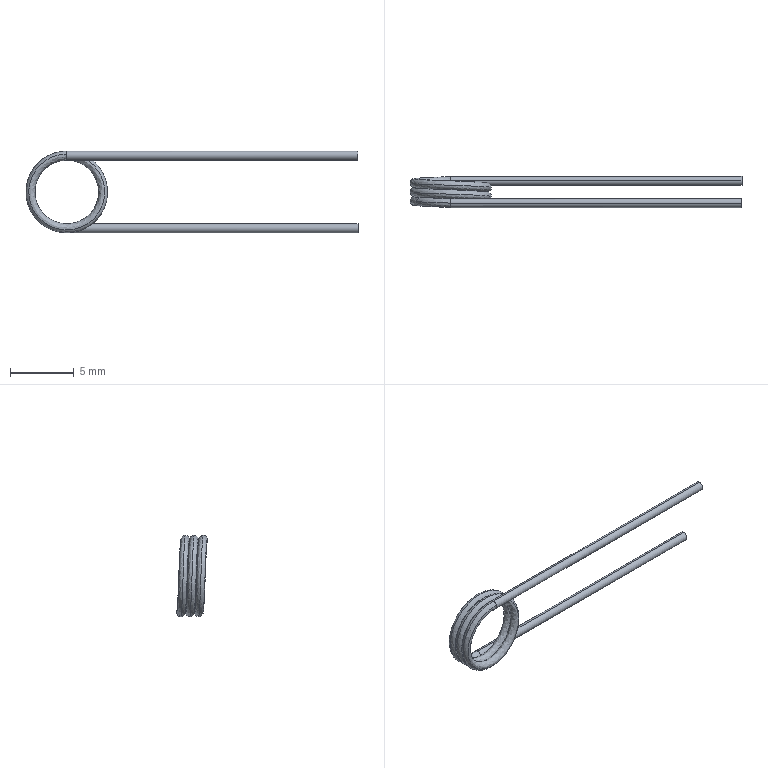Part | SolidWorks | features CompositeCurve 1, Helix 1, MoveFace 1, Sweep 1 | 1 solid | 9 faces | box 26.05 x 2.45 x 6.4 mm | volume 34.304 mm3 | cylinder 4 | spline 3 | plane 2 | commonest cylinder face diameters 0.7 x4
STEP:
#1=CARTESIAN_POINT('',(22.85,1.75,-3.2));
#2=VERTEX_POINT('',#1);
#3=CARTESIAN_POINT('',(22.85,1.75,-2.5));
#4=VERTEX_POINT('',#3);
#5=CARTESIAN_POINT('',(22.85,1.75,-2.85));
#6=DIRECTION('',(1.,0.,0.));
#7=DIRECTION('',(0.,0.00009155,-1.));
#8=AXIS2_PLACEMENT_3D('',#5,#6,#7);
#9=CIRCLE('',#8,0.35);
#10=EDGE_CURVE('',#2,#4,#9,.T.);
#11=ORIENTED_EDGE('',*,*,#10,.F.);
#12=CARTESIAN_POINT('',(-0.000000536,1.75,-3.2));
#13=VERTEX_POINT('',#12);
#14=CARTESIAN_POINT('',(12.85,1.75,-3.2));
#15=DIRECTION('',(-1.,0.,0.));
#16=VECTOR('',#15,1000.);
#17=LINE('',#14,#16);
#18=EDGE_CURVE('',#2,#13,#17,.T.);
#19=ORIENTED_EDGE('',*,*,#18,.T.);
#20=CARTESIAN_POINT('',(-0.006305,2.074,-2.979));
#21=VERTEX_POINT('',#20);
#22=CARTESIAN_POINT('',(0.,1.75,-2.85));
#23=DIRECTION('',(1.,0.,0.));
#24=DIRECTION('',(0.,0.00009155,-1.));
#25=AXIS2_PLACEMENT_3D('',#22,#23,#24);
#26=CIRCLE('',#25,0.35);
#27=EDGE_CURVE('',#13,#21,#26,.T.);
#28=ORIENTED_EDGE('',*,*,#27,.T.);
#29=CARTESIAN_POINT('',(0.,1.75,-2.5));
#30=VERTEX_POINT('',#29);
#31=CARTESIAN_POINT('',(0.,1.75,-2.85));
#32=DIRECTION('',(1.,0.,0.));
#33=DIRECTION('',(0.,0.00009155,-1.));
#34=AXIS2_PLACEMENT_3D('',#31,#32,#33);
#35=CIRCLE('',#34,0.35);
#36=EDGE_CURVE('',#21,#30,#35,.T.);
#37=ORIENTED_EDGE('',*,*,#36,.T.);
#38=CARTESIAN_POINT('',(12.85,1.75,-2.5));
#39=DIRECTION('',(-1.,0.,0.));
#40=VECTOR('',#39,1000.);
#41=LINE('',#38,#40);
#42=EDGE_CURVE('',#4,#30,#41,.T.);
#43=ORIENTED_EDGE('',*,*,#42,.F.);
#44=EDGE_LOOP('',(#11,#19,#28,#37,#43));
#45=FACE_OUTER_BOUND('',#44,.T.);
#46=CARTESIAN_POINT('',(12.85,1.75,-2.85));
#47=DIRECTION('',(-1.,0.,0.));
#48=DIRECTION('',(0.,0.,1.));
#49=AXIS2_PLACEMENT_3D('',#46,#47,#48);
#50=CYLINDRICAL_SURFACE('',#49,0.35);
#51=ADVANCED_FACE('',(#45),#50,.T.);
#52=CARTESIAN_POINT('',(0.006305,0.3239,2.979));
#53=VERTEX_POINT('',#52);
#54=CARTESIAN_POINT('',(0.,0.,3.2));
#55=VERTEX_POINT('',#54);
#56=CARTESIAN_POINT('',(0.006305,0.3239,2.979));
#57=CARTESIAN_POINT('',(0.01048,0.2681,3.104));
#58=CARTESIAN_POINT('',(0.005425,0.1388,3.2));
#59=CARTESIAN_POINT('',(0.,0.,3.2));
#60=B_SPLINE_CURVE_WITH_KNOTS('',3,(#56,#57,#58,#59),.UNSPECIFIED.,.F.,.F.,(4,4),(0.00002721,0.1895),.UNSPECIFIED.);
#61=EDGE_CURVE('',#53,#55,#60,.T.);
#62=ORIENTED_EDGE('',*,*,#61,.T.);
#63=CARTESIAN_POINT('',(22.85,0.,3.2));
#64=VERTEX_POINT('',#63);
#65=CARTESIAN_POINT('',(0.,0.,3.2));
#66=DIRECTION('',(1.,0.,0.));
#67=VECTOR('',#66,1000.);
#68=LINE('',#65,#67);
#69=EDGE_CURVE('',#55,#64,#68,.T.);
#70=ORIENTED_EDGE('',*,*,#69,.T.);
#71=CARTESIAN_POINT('',(22.85,0.,2.5));
#72=VERTEX_POINT('',#71);
#73=CARTESIAN_POINT('',(22.85,0.,2.85));
#74=DIRECTION('',(-1.,0.,0.));
#75=DIRECTION('',(0.,0.,1.));
#76=AXIS2_PLACEMENT_3D('',#73,#74,#75);
#77=CIRCLE('',#76,0.35);
#78=EDGE_CURVE('',#64,#72,#77,.T.);
#79=ORIENTED_EDGE('',*,*,#78,.T.);
#80=CARTESIAN_POINT('',(0.,0.,2.5));
#81=VERTEX_POINT('',#80);
#82=CARTESIAN_POINT('',(0.,0.,2.5));
#83=DIRECTION('',(1.,0.,0.));
#84=VECTOR('',#83,1000.);
#85=LINE('',#82,#84);
#86=EDGE_CURVE('',#81,#72,#85,.T.);
#87=ORIENTED_EDGE('',*,*,#86,.F.);
#88=CARTESIAN_POINT('',(0.,0.,2.85));
#89=DIRECTION('',(-1.,0.,0.));
#90=DIRECTION('',(0.,0.,1.));
#91=AXIS2_PLACEMENT_3D('',#88,#89,#90);
#92=CIRCLE('',#91,0.35);
#93=EDGE_CURVE('',#53,#81,#92,.T.);
#94=ORIENTED_EDGE('',*,*,#93,.F.);
#95=EDGE_LOOP('',(#62,#70,#79,#87,#94));
#96=FACE_OUTER_BOUND('',#95,.T.);
#97=CARTESIAN_POINT('',(0.,0.,2.85));
#98=DIRECTION('',(1.,0.,0.));
#99=DIRECTION('',(0.,0.,-1.));
#100=AXIS2_PLACEMENT_3D('',#97,#98,#99);
#101=CYLINDRICAL_SURFACE('',#100,0.35);
#102=ADVANCED_FACE('',(#96),#101,.T.);
#103=ORIENTED_EDGE('',*,*,#18,.F.);
#104=CARTESIAN_POINT('',(22.85,1.75,-2.85));
#105=DIRECTION('',(1.,0.,0.));
#106=DIRECTION('',(0.,0.00009155,-1.));
#107=AXIS2_PLACEMENT_3D('',#104,#105,#106);
#108=CIRCLE('',#107,0.35);
#109=EDGE_CURVE('',#4,#2,#108,.T.);
#110=ORIENTED_EDGE('',*,*,#109,.F.);
#111=ORIENTED_EDGE('',*,*,#42,.T.);
#112=CARTESIAN_POINT('',(0.006304,1.426,-2.979));
#113=VERTEX_POINT('',#112);
#114=CARTESIAN_POINT('',(0.,1.75,-2.85));
#115=DIRECTION('',(1.,0.,0.));
#116=DIRECTION('',(0.,0.00009155,-1.));
#117=AXIS2_PLACEMENT_3D('',#114,#115,#116);
#118=CIRCLE('',#117,0.35);
#119=EDGE_CURVE('',#30,#113,#118,.T.);
#120=ORIENTED_EDGE('',*,*,#119,.T.);
#121=CARTESIAN_POINT('',(0.,1.75,-2.85));
#122=DIRECTION('',(1.,0.,0.));
#123=DIRECTION('',(0.,0.00009155,-1.));
#124=AXIS2_PLACEMENT_3D('',#121,#122,#123);
#125=CIRCLE('',#124,0.35);
#126=EDGE_CURVE('',#113,#13,#125,.T.);
#127=ORIENTED_EDGE('',*,*,#126,.T.);
#128=EDGE_LOOP('',(#103,#110,#111,#120,#127));
#129=FACE_OUTER_BOUND('',#128,.T.);
#130=CARTESIAN_POINT('',(12.85,1.75,-2.85));
#131=DIRECTION('',(-1.,0.,0.));
#132=DIRECTION('',(0.,0.,1.));
#133=AXIS2_PLACEMENT_3D('',#130,#131,#132);
#134=CYLINDRICAL_SURFACE('',#133,0.35);
#135=ADVANCED_FACE('',(#129),#134,.T.);
#136=ORIENTED_EDGE('',*,*,#36,.F.);
#137=CARTESIAN_POINT('',(0.006305,0.3239,2.979));
#138=CARTESIAN_POINT('',(-0.7712,0.3519,2.981));
#139=CARTESIAN_POINT('',(-1.545,0.381,2.663));
#140=CARTESIAN_POINT('',(-2.649,0.4392,1.566));
#141=CARTESIAN_POINT('',(-2.975,0.4683,0.7939));
#142=CARTESIAN_POINT('',(-2.98,0.5195,-0.5733));
#143=CARTESIAN_POINT('',(-2.806,0.5413,-1.156));
#144=CARTESIAN_POINT('',(-2.162,0.585,-2.13));
#145=CARTESIAN_POINT('',(-1.69,0.6069,-2.521));
#146=CARTESIAN_POINT('',(-0.4324,0.658,-3.048));
#147=CARTESIAN_POINT('',(0.405,0.6871,-3.052));
#148=CARTESIAN_POINT('',(1.67,0.7383,-2.534));
#149=CARTESIAN_POINT('',(2.142,0.7601,-2.15));
#150=CARTESIAN_POINT('',(2.795,0.8037,-1.182));
#151=CARTESIAN_POINT('',(2.976,0.8257,-0.5972));
#152=CARTESIAN_POINT('',(2.981,0.8768,0.7668));
#153=CARTESIAN_POINT('',(2.665,0.9058,1.542));
#154=CARTESIAN_POINT('',(1.702,0.957,2.513));
#155=CARTESIAN_POINT('',(1.167,0.9788,2.801));
#156=CARTESIAN_POINT('',(0.02248,1.022,3.035));
#157=CARTESIAN_POINT('',(-0.587,1.044,2.978));
#158=CARTESIAN_POINT('',(-1.849,1.096,2.461));
#159=CARTESIAN_POINT('',(-2.445,1.125,1.872));
#160=CARTESIAN_POINT('',(-2.973,1.176,0.6109));
#161=CARTESIAN_POINT('',(-3.035,1.198,0.005944));
#162=CARTESIAN_POINT('',(-2.812,1.241,-1.14));
#163=CARTESIAN_POINT('',(-2.526,1.263,-1.682));
#164=CARTESIAN_POINT('',(-1.566,1.314,-2.65));
#165=CARTESIAN_POINT('',(-0.7938,1.343,-2.975));
#166=CARTESIAN_POINT('',(0.5733,1.395,-2.98));
#167=CARTESIAN_POINT('',(1.156,1.416,-2.806));
#168=CARTESIAN_POINT('',(2.13,1.46,-2.162));
#169=CARTESIAN_POINT('',(2.521,1.482,-1.69));
#170=CARTESIAN_POINT('',(3.048,1.533,-0.4324));
#171=CARTESIAN_POINT('',(3.052,1.562,0.405));
#172=CARTESIAN_POINT('',(2.534,1.613,1.67));
#173=CARTESIAN_POINT('',(2.15,1.635,2.142));
#174=CARTESIAN_POINT('',(1.182,1.679,2.795));
#175=CARTESIAN_POINT('',(0.5972,1.701,2.976));
#176=CARTESIAN_POINT('',(-0.7668,1.752,2.981));
#177=CARTESIAN_POINT('',(-1.542,1.781,2.665));
#178=CARTESIAN_POINT('',(-2.513,1.832,1.702));
#179=CARTESIAN_POINT('',(-2.801,1.854,1.167));
#180=CARTESIAN_POINT('',(-3.034,1.897,0.0225));
#181=CARTESIAN_POINT('',(-2.978,1.919,-0.587));
#182=CARTESIAN_POINT('',(-2.46,1.971,-1.85));
#183=CARTESIAN_POINT('',(-1.872,2.,-2.445));
#184=CARTESIAN_POINT('',(-0.7917,2.043,-2.897));
#185=CARTESIAN_POINT('',(-0.4042,2.058,-2.976));
#186=CARTESIAN_POINT('',(-0.006305,2.074,-2.979));
#187=B_SPLINE_CURVE_WITH_KNOTS('',3,(#137,#138,#139,#140,#141,#142,#143,#144,#145,#146,#147,#148,#149,#150,#151,#152,#153,#154,#155,#156,#157,#158,#159,#160,#161,#162,#163,#164,#165,#166,#167,#168,#169,#170,#171,#172,#173,#174,#175,#176,#177,#178,#179,#180,#181,#182,#183,#184,#185,#186),.UNSPECIFIED.,.F.,.F.,(4,2,2,2,2,2,2,2,2,2,2,2,2,2,2,2,2,2,2,2,2,2,2,2,4),(0.,0.04998,0.09999,0.1375,0.175,0.225,0.2625,0.3,0.35,0.3875,0.425,0.475,0.5125,0.55,0.6,0.6375,0.675,0.725,0.7625,0.8,0.85,0.8875,0.925,0.975,1.),.UNSPECIFIED.);
#188=EDGE_CURVE('',#53,#21,#187,.T.);
#189=ORIENTED_EDGE('',*,*,#188,.F.);
#190=ORIENTED_EDGE('',*,*,#93,.T.);
#191=CARTESIAN_POINT('',(-0.006304,-0.3239,2.979));
#192=VERTEX_POINT('',#191);
#193=CARTESIAN_POINT('',(0.,0.,2.85));
#194=DIRECTION('',(-1.,0.,0.));
#195=DIRECTION('',(0.,0.,1.));
#196=AXIS2_PLACEMENT_3D('',#193,#194,#195);
#197=CIRCLE('',#196,0.35);
#198=EDGE_CURVE('',#81,#192,#197,.T.);
#199=ORIENTED_EDGE('',*,*,#198,.T.);
#200=CARTESIAN_POINT('',(0.006304,1.426,-2.979));
#201=CARTESIAN_POINT('',(-0.379,1.413,-2.98));
#202=CARTESIAN_POINT('',(-0.7673,1.398,-2.904));
#203=CARTESIAN_POINT('',(-1.851,1.354,-2.461));
#204=CARTESIAN_POINT('',(-2.445,1.325,-1.871));
#205=CARTESIAN_POINT('',(-2.973,1.274,-0.6122));
#206=CARTESIAN_POINT('',(-3.035,1.252,-0.003211));
#207=CARTESIAN_POINT('',(-2.811,1.209,1.143));
#208=CARTESIAN_POINT('',(-2.527,1.187,1.681));
#209=CARTESIAN_POINT('',(-1.565,1.136,2.652));
#210=CARTESIAN_POINT('',(-0.792,1.107,2.975));
#211=CARTESIAN_POINT('',(0.572,1.056,2.981));
#212=CARTESIAN_POINT('',(1.158,1.034,2.805));
#213=CARTESIAN_POINT('',(2.132,0.99,2.16));
#214=CARTESIAN_POINT('',(2.52,0.9682,1.692));
#215=CARTESIAN_POINT('',(3.049,0.917,0.4308));
#216=CARTESIAN_POINT('',(3.052,0.8879,-0.4067));
#217=CARTESIAN_POINT('',(2.535,0.8368,-1.669));
#218=CARTESIAN_POINT('',(2.148,0.8149,-2.144));
#219=CARTESIAN_POINT('',(1.18,0.7712,-2.796));
#220=CARTESIAN_POINT('',(0.5985,0.7494,-2.976));
#221=CARTESIAN_POINT('',(-0.7686,0.6982,-2.981));
#222=CARTESIAN_POINT('',(-1.544,0.6692,-2.664));
#223=CARTESIAN_POINT('',(-2.512,0.6181,-1.703));
#224=CARTESIAN_POINT('',(-2.802,0.5961,-1.164));
#225=CARTESIAN_POINT('',(-3.035,0.5525,-0.01977));
#226=CARTESIAN_POINT('',(-2.978,0.5307,0.5858));
#227=CARTESIAN_POINT('',(-2.46,0.4795,1.851));
#228=CARTESIAN_POINT('',(-1.87,0.4504,2.445));
#229=CARTESIAN_POINT('',(-0.6122,0.3993,2.973));
#230=CARTESIAN_POINT('',(-0.003226,0.3774,3.035));
#231=CARTESIAN_POINT('',(1.143,0.3337,2.811));
#232=CARTESIAN_POINT('',(1.681,0.3119,2.527));
#233=CARTESIAN_POINT('',(2.652,0.2607,1.565));
#234=CARTESIAN_POINT('',(2.975,0.2317,0.792));
#235=CARTESIAN_POINT('',(2.981,0.1806,-0.572));
#236=CARTESIAN_POINT('',(2.805,0.1586,-1.158));
#237=CARTESIAN_POINT('',(2.16,0.115,-2.132));
#238=CARTESIAN_POINT('',(1.692,0.09317,-2.52));
#239=CARTESIAN_POINT('',(0.4308,0.04196,-3.049));
#240=CARTESIAN_POINT('',(-0.4067,0.01292,-3.052));
#241=CARTESIAN_POINT('',(-1.669,-0.03818,-2.535));
#242=CARTESIAN_POINT('',(-2.144,-0.06013,-2.148));
#243=CARTESIAN_POINT('',(-2.796,-0.1038,-1.18));
#244=CARTESIAN_POINT('',(-2.976,-0.1256,-0.5985));
#245=CARTESIAN_POINT('',(-2.981,-0.1768,0.7687));
#246=CARTESIAN_POINT('',(-2.663,-0.2059,1.544));
#247=CARTESIAN_POINT('',(-1.567,-0.2642,2.65));
#248=CARTESIAN_POINT('',(-0.7966,-0.2932,2.975));
#249=CARTESIAN_POINT('',(-0.006304,-0.3239,2.979));
#250=B_SPLINE_CURVE_WITH_KNOTS('',3,(#200,#201,#202,#203,#204,#205,#206,#207,#208,#209,#210,#211,#212,#213,#214,#215,#216,#217,#218,#219,#220,#221,#222,#223,#224,#225,#226,#227,#228,#229,#230,#231,#232,#233,#234,#235,#236,#237,#238,#239,#240,#241,#242,#243,#244,#245,#246,#247,#248,#249),.UNSPECIFIED.,.F.,.F.,(4,2,2,2,2,2,2,2,2,2,2,2,2,2,2,2,2,2,2,2,2,2,2,2,4),(0.,0.02496,0.07501,0.1125,0.15,0.2,0.2375,0.275,0.325,0.3625,0.4,0.45,0.4875,0.525,0.575,0.6125,0.65,0.7,0.7375,0.775,0.825,0.8625,0.9,0.95,1.),.UNSPECIFIED.);
#251=EDGE_CURVE('',#113,#192,#250,.T.);
#252=ORIENTED_EDGE('',*,*,#251,.F.);
#253=ORIENTED_EDGE('',*,*,#119,.F.);
#254=EDGE_LOOP('',(#136,#189,#190,#199,#252,#253));
#255=FACE_OUTER_BOUND('',#254,.T.);
#256=CARTESIAN_POINT('',(-0.01261,2.073,-2.978));
#257=CARTESIAN_POINT('',(-0.9931,2.036,-2.974));
#258=CARTESIAN_POINT('',(-1.942,2.,-2.452));
#259=CARTESIAN_POINT('',(-3.022,1.927,-0.8338));
#260=CARTESIAN_POINT('',(-3.123,1.89,0.2539));
#261=CARTESIAN_POINT('',(-2.369,1.817,2.048));
#262=CARTESIAN_POINT('',(-1.523,1.781,2.732));
#263=CARTESIAN_POINT('',(0.3864,1.708,3.111));
#264=CARTESIAN_POINT('',(1.43,1.671,2.788));
#265=CARTESIAN_POINT('',(2.798,1.599,1.405));
#266=CARTESIAN_POINT('',(3.107,1.562,0.3615));
#267=CARTESIAN_POINT('',(2.726,1.489,-1.547));
#268=CARTESIAN_POINT('',(2.029,1.453,-2.388));
#269=CARTESIAN_POINT('',(0.2273,1.38,-3.123));
#270=CARTESIAN_POINT('',(-0.8551,1.343,-3.009));
#271=CARTESIAN_POINT('',(-2.473,1.271,-1.927));
#272=CARTESIAN_POINT('',(-2.982,1.234,-0.9604));
#273=CARTESIAN_POINT('',(-2.972,1.161,0.9852));
#274=CARTESIAN_POINT('',(-2.453,1.125,1.942));
#275=CARTESIAN_POINT('',(-0.8335,1.052,3.022));
#276=CARTESIAN_POINT('',(0.2539,1.015,3.123));
#277=CARTESIAN_POINT('',(2.048,0.9425,2.369));
#278=CARTESIAN_POINT('',(2.732,0.9059,1.523));
#279=CARTESIAN_POINT('',(3.111,0.8331,-0.3864));
#280=CARTESIAN_POINT('',(2.788,0.7965,-1.43));
#281=CARTESIAN_POINT('',(1.405,0.7237,-2.798));
#282=CARTESIAN_POINT('',(0.3615,0.6872,-3.107));
#283=CARTESIAN_POINT('',(-1.547,0.6143,-2.726));
#284=CARTESIAN_POINT('',(-2.388,0.5777,-2.029));
#285=CARTESIAN_POINT('',(-3.123,0.505,-0.2273));
#286=CARTESIAN_POINT('',(-3.009,0.4684,0.8554));
#287=CARTESIAN_POINT('',(-1.927,0.3956,2.473));
#288=CARTESIAN_POINT('',(-0.9676,0.3593,2.982));
#289=CARTESIAN_POINT('',(0.01261,0.3226,2.978));
#290=CARTESIAN_POINT('',(-0.0161,2.162,-2.771));
#291=CARTESIAN_POINT('',(-0.9269,2.125,-2.766));
#292=CARTESIAN_POINT('',(-1.811,2.089,-2.279));
#293=CARTESIAN_POINT('',(-2.813,2.016,-0.7712));
#294=CARTESIAN_POINT('',(-2.906,1.979,0.2409));
#295=CARTESIAN_POINT('',(-2.201,1.907,1.909));
#296=CARTESIAN_POINT('',(-1.413,1.87,2.545));
#297=CARTESIAN_POINT('',(0.3644,1.797,2.894));
#298=CARTESIAN_POINT('',(1.334,1.761,2.592));
#299=CARTESIAN_POINT('',(2.606,1.688,1.303));
#300=CARTESIAN_POINT('',(2.892,1.651,0.3318));
#301=CARTESIAN_POINT('',(2.535,1.579,-1.444));
#302=CARTESIAN_POINT('',(1.884,1.542,-2.225));
#303=CARTESIAN_POINT('',(0.2064,1.469,-2.907));
#304=CARTESIAN_POINT('',(-0.8001,1.433,-2.799));
#305=CARTESIAN_POINT('',(-2.304,1.36,-1.789));
#306=CARTESIAN_POINT('',(-2.777,1.323,-0.8894));
#307=CARTESIAN_POINT('',(-2.764,1.25,0.9216));
#308=CARTESIAN_POINT('',(-2.279,1.214,1.81));
#309=CARTESIAN_POINT('',(-0.771,1.141,2.814));
#310=CARTESIAN_POINT('',(0.2409,1.104,2.906));
#311=CARTESIAN_POINT('',(1.909,1.032,2.201));
#312=CARTESIAN_POINT('',(2.545,0.9951,1.413));
#313=CARTESIAN_POINT('',(2.894,0.9223,-0.3644));
#314=CARTESIAN_POINT('',(2.592,0.8857,-1.334));
#315=CARTESIAN_POINT('',(1.303,0.8129,-2.606));
#316=CARTESIAN_POINT('',(0.3318,0.7764,-2.892));
#317=CARTESIAN_POINT('',(-1.444,0.7035,-2.535));
#318=CARTESIAN_POINT('',(-2.225,0.667,-1.884));
#319=CARTESIAN_POINT('',(-2.907,0.5942,-0.2064));
#320=CARTESIAN_POINT('',(-2.798,0.5576,0.8003));
#321=CARTESIAN_POINT('',(-1.789,0.4848,2.304));
#322=CARTESIAN_POINT('',(-0.8958,0.4485,2.776));
#323=CARTESIAN_POINT('',(0.0161,0.4118,2.771));
#324=CARTESIAN_POINT('',(-0.008888,1.977,-2.5));
#325=CARTESIAN_POINT('',(-0.8283,1.941,-2.497));
#326=CARTESIAN_POINT('',(-1.629,1.904,-2.059));
#327=CARTESIAN_POINT('',(-2.536,1.832,-0.7012));
#328=CARTESIAN_POINT('',(-2.622,1.795,0.2114));
#329=CARTESIAN_POINT('',(-1.989,1.722,1.718));
#330=CARTESIAN_POINT('',(-1.28,1.686,2.292));
#331=CARTESIAN_POINT('',(0.3232,1.613,2.612));
#332=CARTESIAN_POINT('',(1.199,1.576,2.341));
#333=CARTESIAN_POINT('',(2.349,1.503,1.18));
#334=CARTESIAN_POINT('',(2.608,1.467,0.3051));
#335=CARTESIAN_POINT('',(2.29,1.394,-1.298));
#336=CARTESIAN_POINT('',(1.704,1.358,-2.003));
#337=CARTESIAN_POINT('',(0.1914,1.285,-2.622));
#338=CARTESIAN_POINT('',(-0.716,1.248,-2.526));
#339=CARTESIAN_POINT('',(-2.075,1.175,-1.618));
#340=CARTESIAN_POINT('',(-2.503,1.139,-0.808));
#341=CARTESIAN_POINT('',(-2.495,1.066,0.8264));
#342=CARTESIAN_POINT('',(-2.06,1.029,1.628));
#343=CARTESIAN_POINT('',(-0.701,0.9565,2.537));
#344=CARTESIAN_POINT('',(0.2114,0.92,2.622));
#345=CARTESIAN_POINT('',(1.718,0.8471,1.989));
#346=CARTESIAN_POINT('',(2.292,0.8107,1.28));
#347=CARTESIAN_POINT('',(2.612,0.7378,-0.3232));
#348=CARTESIAN_POINT('',(2.341,0.7013,-1.199));
#349=CARTESIAN_POINT('',(1.18,0.6284,-2.349));
#350=CARTESIAN_POINT('',(0.3051,0.5919,-2.608));
#351=CARTESIAN_POINT('',(-1.298,0.519,-2.29));
#352=CARTESIAN_POINT('',(-2.003,0.4825,-1.704));
#353=CARTESIAN_POINT('',(-2.622,0.4096,-0.1914));
#354=CARTESIAN_POINT('',(-2.525,0.3732,0.7162));
#355=CARTESIAN_POINT('',(-1.619,0.3003,2.075));
#356=CARTESIAN_POINT('',(-0.8134,0.2639,2.503));
#357=CARTESIAN_POINT('',(0.008889,0.2274,2.5));
#358=CARTESIAN_POINT('',(0.008895,1.522,-2.5));
#359=CARTESIAN_POINT('',(-0.8105,1.486,-2.503));
#360=CARTESIAN_POINT('',(-1.614,1.45,-2.071));
#361=CARTESIAN_POINT('',(-2.532,1.377,-0.7193));
#362=CARTESIAN_POINT('',(-2.623,1.34,0.1927));
#363=CARTESIAN_POINT('',(-2.001,1.267,1.704));
#364=CARTESIAN_POINT('',(-1.296,1.231,2.283));
#365=CARTESIAN_POINT('',(0.3046,1.158,2.614));
#366=CARTESIAN_POINT('',(1.182,1.121,2.35));
#367=CARTESIAN_POINT('',(2.341,1.048,1.197));
#368=CARTESIAN_POINT('',(2.606,1.012,0.3236));
#369=CARTESIAN_POINT('',(2.299,0.9391,-1.282));
#370=CARTESIAN_POINT('',(1.719,0.9026,-1.991));
#371=CARTESIAN_POINT('',(0.2101,0.8297,-2.62));
#372=CARTESIAN_POINT('',(-0.6981,0.7933,-2.531));
#373=CARTESIAN_POINT('',(-2.064,0.7204,-1.633));
#374=CARTESIAN_POINT('',(-2.497,0.6839,-0.8259));
#375=CARTESIAN_POINT('',(-2.501,0.611,0.8087));
#376=CARTESIAN_POINT('',(-2.071,0.5745,1.614));
#377=CARTESIAN_POINT('',(-0.7191,0.5016,2.532));
#378=CARTESIAN_POINT('',(0.1927,0.4651,2.623));
#379=CARTESIAN_POINT('',(1.704,0.3922,2.001));
#380=CARTESIAN_POINT('',(2.283,0.3558,1.296));
#381=CARTESIAN_POINT('',(2.614,0.2829,-0.3046));
#382=CARTESIAN_POINT('',(2.35,0.2464,-1.182));
#383=CARTESIAN_POINT('',(1.197,0.1735,-2.341));
#384=CARTESIAN_POINT('',(0.3236,0.137,-2.606));
#385=CARTESIAN_POINT('',(-1.282,0.0641,-2.299));
#386=CARTESIAN_POINT('',(-1.991,0.02763,-1.719));
#387=CARTESIAN_POINT('',(-2.62,-0.04528,-0.2101));
#388=CARTESIAN_POINT('',(-2.531,-0.08173,0.6983));
#389=CARTESIAN_POINT('',(-1.633,-0.1546,2.064));
#390=CARTESIAN_POINT('',(-0.8313,-0.191,2.497));
#391=CARTESIAN_POINT('',(-0.008894,-0.2275,2.5));
#392=CARTESIAN_POINT('',(0.0161,1.338,-2.771));
#393=CARTESIAN_POINT('',(-0.8947,1.302,-2.777));
#394=CARTESIAN_POINT('',(-1.785,1.265,-2.3));
#395=CARTESIAN_POINT('',(-2.804,1.192,-0.804));
#396=CARTESIAN_POINT('',(-2.908,1.156,0.2071));
#397=CARTESIAN_POINT('',(-2.223,1.083,1.884));
#398=CARTESIAN_POINT('',(-1.443,1.046,2.528));
#399=CARTESIAN_POINT('',(0.3307,0.9736,2.899));
#400=CARTESIAN_POINT('',(1.304,0.937,2.608));
#401=CARTESIAN_POINT('',(2.591,0.8642,1.333));
#402=CARTESIAN_POINT('',(2.888,0.8277,0.3653));
#403=CARTESIAN_POINT('',(2.552,0.7548,-1.415));
#404=CARTESIAN_POINT('',(1.91,0.7183,-2.203));
#405=CARTESIAN_POINT('',(0.2402,0.6455,-2.904));
#406=CARTESIAN_POINT('',(-0.7677,0.6089,-2.808));
#407=CARTESIAN_POINT('',(-2.284,0.5361,-1.816));
#408=CARTESIAN_POINT('',(-2.766,0.4995,-0.9217));
#409=CARTESIAN_POINT('',(-2.775,0.4267,0.8895));
#410=CARTESIAN_POINT('',(-2.3,0.3902,1.784));
#411=CARTESIAN_POINT('',(-0.8038,0.3173,2.805));
#412=CARTESIAN_POINT('',(0.2071,0.2808,2.908));
#413=CARTESIAN_POINT('',(1.884,0.208,2.223));
#414=CARTESIAN_POINT('',(2.528,0.1714,1.443));
#415=CARTESIAN_POINT('',(2.899,0.09857,-0.3307));
#416=CARTESIAN_POINT('',(2.608,0.06204,-1.304));
#417=CARTESIAN_POINT('',(1.333,-0.01079,-2.591));
#418=CARTESIAN_POINT('',(0.3653,-0.0473,-2.888));
#419=CARTESIAN_POINT('',(-1.415,-0.1202,-2.552));
#420=CARTESIAN_POINT('',(-2.203,-0.1567,-1.91));
#421=CARTESIAN_POINT('',(-2.904,-0.2295,-0.2402));
#422=CARTESIAN_POINT('',(-2.807,-0.2661,0.7679));
#423=CARTESIAN_POINT('',(-1.816,-0.3389,2.283));
#424=CARTESIAN_POINT('',(-0.9282,-0.3752,2.766));
#425=CARTESIAN_POINT('',(-0.0161,-0.4119,2.771));
#426=CARTESIAN_POINT('',(0.01261,1.427,-2.978));
#427=CARTESIAN_POINT('',(-0.9679,1.391,-2.982));
#428=CARTESIAN_POINT('',(-1.922,1.354,-2.469));
#429=CARTESIAN_POINT('',(-3.015,1.282,-0.8595));
#430=CARTESIAN_POINT('',(-3.125,1.245,0.2275));
#431=CARTESIAN_POINT('',(-2.386,1.172,2.028));
#432=CARTESIAN_POINT('',(-1.546,1.136,2.72));
#433=CARTESIAN_POINT('',(0.36,1.063,3.114));
#434=CARTESIAN_POINT('',(1.406,1.026,2.8));
#435=CARTESIAN_POINT('',(2.787,0.9536,1.429));
#436=CARTESIAN_POINT('',(3.104,0.917,0.3878));
#437=CARTESIAN_POINT('',(2.739,0.8442,-1.524));
#438=CARTESIAN_POINT('',(2.049,0.8076,-2.37));
#439=CARTESIAN_POINT('',(0.2537,0.7349,-3.121));
#440=CARTESIAN_POINT('',(-0.8297,0.6983,-3.016));
#441=CARTESIAN_POINT('',(-2.457,0.6254,-1.948));
#442=CARTESIAN_POINT('',(-2.974,0.5889,-0.9857));
#443=CARTESIAN_POINT('',(-2.981,0.5161,0.96));
#444=CARTESIAN_POINT('',(-2.469,0.4795,1.921));
#445=CARTESIAN_POINT('',(-0.8592,0.4067,3.015));
#446=CARTESIAN_POINT('',(0.2275,0.3701,3.125));
#447=CARTESIAN_POINT('',(2.028,0.2974,2.386));
#448=CARTESIAN_POINT('',(2.72,0.2608,1.546));
#449=CARTESIAN_POINT('',(3.114,0.1879,-0.36));
#450=CARTESIAN_POINT('',(2.8,0.1514,-1.406));
#451=CARTESIAN_POINT('',(1.429,0.07861,-2.787));
#452=CARTESIAN_POINT('',(0.3878,0.04204,-3.104));
#453=CARTESIAN_POINT('',(-1.524,-0.03081,-2.739));
#454=CARTESIAN_POINT('',(-2.371,-0.06738,-2.049));
#455=CARTESIAN_POINT('',(-3.121,-0.1401,-0.2537));
#456=CARTESIAN_POINT('',(-3.016,-0.1767,0.83));
#457=CARTESIAN_POINT('',(-1.948,-0.2496,2.456));
#458=CARTESIAN_POINT('',(-0.993,-0.2858,2.974));
#459=CARTESIAN_POINT('',(-0.01261,-0.3225,2.978));
#460=B_SPLINE_SURFACE_WITH_KNOTS('',3,3,((#256,#257,#258,#259,#260,#261,#262,#263,#264,#265,#266,#267,#268,#269,#270,#271,#272,#273,#274,#275,#276,#277,#278,#279,#280,#281,#282,#283,#284,#285,#286,#287,#288,#289),(#290,#291,#292,#293,#294,#295,#296,#297,#298,#299,#300,#301,#302,#303,#304,#305,#306,#307,#308,#309,#310,#311,#312,#313,#314,#315,#316,#317,#318,#319,#320,#321,#322,#323),(#324,#325,#326,#327,#328,#329,#330,#331,#332,#333,#334,#335,#336,#337,#338,#339,#340,#341,#342,#343,#344,#345,#346,#347,#348,#349,#350,#351,#352,#353,#354,#355,#356,#357),(#358,#359,#360,#361,#362,#363,#364,#365,#366,#367,#368,#369,#370,#371,#372,#373,#374,#375,#376,#377,#378,#379,#380,#381,#382,#383,#384,#385,#386,#387,#388,#389,#390,#391),(#392,#393,#394,#395,#396,#397,#398,#399,#400,#401,#402,#403,#404,#405,#406,#407,#408,#409,#410,#411,#412,#413,#414,#415,#416,#417,#418,#419,#420,#421,#422,#423,#424,#425),(#426,#427,#428,#429,#430,#431,#432,#433,#434,#435,#436,#437,#438,#439,#440,#441,#442,#443,#444,#445,#446,#447,#448,#449,#450,#451,#452,#453,#454,#455,#456,#457,#458,#459)),.UNSPECIFIED.,.F.,.F.,.F.,(4,2,4),(4,2,2,2,2,2,2,2,2,2,2,2,2,2,2,2,4),(0.1895,0.5,0.8106),(0.,0.0625,0.125,0.1875,0.25,0.3125,0.375,0.4375,0.5,0.5625,0.625,0.6875,0.75,0.8125,0.875,0.9375,1.),.UNSPECIFIED.);
#461=ADVANCED_FACE('',(#255),#460,.F.);
#462=ORIENTED_EDGE('',*,*,#126,.F.);
#463=ORIENTED_EDGE('',*,*,#251,.T.);
#464=CARTESIAN_POINT('',(0.,0.,3.2));
#465=CARTESIAN_POINT('',(-0.005423,-0.1387,3.2));
#466=CARTESIAN_POINT('',(-0.01048,-0.268,3.104));
#467=CARTESIAN_POINT('',(-0.006304,-0.3239,2.979));
#468=B_SPLINE_CURVE_WITH_KNOTS('',3,(#464,#465,#466,#467),.UNSPECIFIED.,.F.,.F.,(4,4),(0.8106,1.),.UNSPECIFIED.);
#469=EDGE_CURVE('',#55,#192,#468,.T.);
#470=ORIENTED_EDGE('',*,*,#469,.F.);
#471=CARTESIAN_POINT('',(-0.000000536,1.75,-3.2));
#472=CARTESIAN_POINT('',(-0.4215,1.735,-3.2));
#473=CARTESIAN_POINT('',(-0.8371,1.721,-3.117));
#474=CARTESIAN_POINT('',(-2.001,1.677,-2.635));
#475=CARTESIAN_POINT('',(-2.635,1.648,-2.));
#476=CARTESIAN_POINT('',(-3.197,1.597,-0.6438));
#477=CARTESIAN_POINT('',(-3.261,1.575,0.01064));
#478=CARTESIAN_POINT('',(-3.015,1.531,1.241));
#479=CARTESIAN_POINT('',(-2.708,1.51,1.817));
#480=CARTESIAN_POINT('',(-1.669,1.458,2.857));
#481=CARTESIAN_POINT('',(-0.8382,1.429,3.2));
#482=CARTESIAN_POINT('',(0.6287,1.378,3.2));
#483=CARTESIAN_POINT('',(1.258,1.356,3.008));
#484=CARTESIAN_POINT('',(2.3,1.313,2.311));
#485=CARTESIAN_POINT('',(2.715,1.291,1.807));
#486=CARTESIAN_POINT('',(3.278,1.239,0.4484));
#487=CARTESIAN_POINT('',(3.277,1.211,-0.4502));
#488=CARTESIAN_POINT('',(2.716,1.159,-1.805));
#489=CARTESIAN_POINT('',(2.298,1.137,-2.313));
#490=CARTESIAN_POINT('',(1.255,1.094,-3.01));
#491=CARTESIAN_POINT('',(0.6301,1.072,-3.2));
#492=CARTESIAN_POINT('',(-0.8402,1.021,-3.2));
#493=CARTESIAN_POINT('',(-1.67,0.9918,-2.855));
#494=CARTESIAN_POINT('',(-2.707,0.9406,-1.818));
#495=CARTESIAN_POINT('',(-3.017,0.9186,-1.238));
#496=CARTESIAN_POINT('',(-3.261,0.875,-0.007701));
#497=CARTESIAN_POINT('',(-3.198,0.8533,0.6424));
#498=CARTESIAN_POINT('',(-2.635,0.8019,2.001));
#499=CARTESIAN_POINT('',(-1.999,0.773,2.636));
#500=CARTESIAN_POINT('',(-0.6438,0.7218,3.197));
#501=CARTESIAN_POINT('',(0.01062,0.6999,3.261));
#502=CARTESIAN_POINT('',(1.241,0.6563,3.015));
#503=CARTESIAN_POINT('',(1.817,0.6345,2.708));
#504=CARTESIAN_POINT('',(2.857,0.5832,1.669));
#505=CARTESIAN_POINT('',(3.2,0.5543,0.8382));
#506=CARTESIAN_POINT('',(3.2,0.5031,-0.6287));
#507=CARTESIAN_POINT('',(3.008,0.4811,-1.258));
#508=CARTESIAN_POINT('',(2.311,0.4375,-2.3));
#509=CARTESIAN_POINT('',(1.807,0.4158,-2.715));
#510=CARTESIAN_POINT('',(0.4484,0.3644,-3.278));
#511=CARTESIAN_POINT('',(-0.4502,0.3355,-3.277));
#512=CARTESIAN_POINT('',(-1.805,0.2843,-2.716));
#513=CARTESIAN_POINT('',(-2.313,0.2624,-2.298));
#514=CARTESIAN_POINT('',(-3.01,0.2188,-1.255));
#515=CARTESIAN_POINT('',(-3.2,0.197,-0.6301));
#516=CARTESIAN_POINT('',(-3.2,0.1457,0.8403));
#517=CARTESIAN_POINT('',(-2.854,0.1167,1.671));
#518=CARTESIAN_POINT('',(-1.671,0.05831,2.854));
#519=CARTESIAN_POINT('',(-0.8425,0.02943,3.2));
#520=CARTESIAN_POINT('',(0.,0.,3.2));
#521=B_SPLINE_CURVE_WITH_KNOTS('',3,(#471,#472,#473,#474,#475,#476,#477,#478,#479,#480,#481,#482,#483,#484,#485,#486,#487,#488,#489,#490,#491,#492,#493,#494,#495,#496,#497,#498,#499,#500,#501,#502,#503,#504,#505,#506,#507,#508,#509,#510,#511,#512,#513,#514,#515,#516,#517,#518,#519,#520),.UNSPECIFIED.,.F.,.F.,(4,2,2,2,2,2,2,2,2,2,2,2,2,2,2,2,2,2,2,2,2,2,2,2,4),(0.,0.02496,0.07501,0.1125,0.15,0.2,0.2375,0.275,0.325,0.3625,0.4,0.45,0.4875,0.525,0.575,0.6125,0.65,0.7,0.7375,0.775,0.825,0.8625,0.9,0.95,1.),.UNSPECIFIED.);
#522=EDGE_CURVE('',#13,#55,#521,.T.);
#523=ORIENTED_EDGE('',*,*,#522,.F.);
#524=EDGE_LOOP('',(#462,#463,#470,#523));
#525=FACE_OUTER_BOUND('',#524,.T.);
#526=CARTESIAN_POINT('',(0.01261,1.427,-2.978));
#527=CARTESIAN_POINT('',(-0.379,1.413,-2.98));
#528=CARTESIAN_POINT('',(-0.7673,1.398,-2.904));
#529=CARTESIAN_POINT('',(-1.851,1.354,-2.461));
#530=CARTESIAN_POINT('',(-2.445,1.325,-1.871));
#531=CARTESIAN_POINT('',(-2.973,1.274,-0.6122));
#532=CARTESIAN_POINT('',(-3.035,1.252,-0.003211));
#533=CARTESIAN_POINT('',(-2.811,1.209,1.143));
#534=CARTESIAN_POINT('',(-2.527,1.187,1.681));
#535=CARTESIAN_POINT('',(-1.565,1.136,2.652));
#536=CARTESIAN_POINT('',(-0.792,1.107,2.975));
#537=CARTESIAN_POINT('',(0.572,1.056,2.981));
#538=CARTESIAN_POINT('',(1.158,1.034,2.805));
#539=CARTESIAN_POINT('',(2.132,0.99,2.16));
#540=CARTESIAN_POINT('',(2.52,0.9682,1.692));
#541=CARTESIAN_POINT('',(3.049,0.917,0.4308));
#542=CARTESIAN_POINT('',(3.052,0.8879,-0.4067));
#543=CARTESIAN_POINT('',(2.535,0.8368,-1.669));
#544=CARTESIAN_POINT('',(2.148,0.8149,-2.144));
#545=CARTESIAN_POINT('',(1.18,0.7712,-2.796));
#546=CARTESIAN_POINT('',(0.5985,0.7494,-2.976));
#547=CARTESIAN_POINT('',(-0.7686,0.6982,-2.981));
#548=CARTESIAN_POINT('',(-1.544,0.6692,-2.664));
#549=CARTESIAN_POINT('',(-2.512,0.6181,-1.703));
#550=CARTESIAN_POINT('',(-2.802,0.5961,-1.164));
#551=CARTESIAN_POINT('',(-3.035,0.5525,-0.01977));
#552=CARTESIAN_POINT('',(-2.978,0.5307,0.5858));
#553=CARTESIAN_POINT('',(-2.46,0.4795,1.851));
#554=CARTESIAN_POINT('',(-1.87,0.4504,2.445));
#555=CARTESIAN_POINT('',(-0.6122,0.3993,2.973));
#556=CARTESIAN_POINT('',(-0.003226,0.3774,3.035));
#557=CARTESIAN_POINT('',(1.143,0.3337,2.811));
#558=CARTESIAN_POINT('',(1.681,0.3119,2.527));
#559=CARTESIAN_POINT('',(2.652,0.2607,1.565));
#560=CARTESIAN_POINT('',(2.975,0.2317,0.792));
#561=CARTESIAN_POINT('',(2.981,0.1806,-0.572));
#562=CARTESIAN_POINT('',(2.805,0.1586,-1.158));
#563=CARTESIAN_POINT('',(2.16,0.115,-2.132));
#564=CARTESIAN_POINT('',(1.692,0.09317,-2.52));
#565=CARTESIAN_POINT('',(0.4308,0.04196,-3.049));
#566=CARTESIAN_POINT('',(-0.4067,0.01292,-3.052));
#567=CARTESIAN_POINT('',(-1.669,-0.03818,-2.535));
#568=CARTESIAN_POINT('',(-2.144,-0.06013,-2.148));
#569=CARTESIAN_POINT('',(-2.796,-0.1038,-1.18));
#570=CARTESIAN_POINT('',(-2.976,-0.1256,-0.5985));
#571=CARTESIAN_POINT('',(-2.981,-0.1768,0.7687));
#572=CARTESIAN_POINT('',(-2.663,-0.2059,1.544));
#573=CARTESIAN_POINT('',(-1.567,-0.2642,2.65));
#574=CARTESIAN_POINT('',(-0.7966,-0.2932,2.975));
#575=CARTESIAN_POINT('',(-0.01261,-0.3225,2.978));
#576=CARTESIAN_POINT('',(0.01048,1.482,-3.104));
#577=CARTESIAN_POINT('',(-0.3981,1.467,-3.106));
#578=CARTESIAN_POINT('',(-0.802,1.453,-3.026));
#579=CARTESIAN_POINT('',(-1.932,1.409,-2.563));
#580=CARTESIAN_POINT('',(-2.55,1.38,-1.948));
#581=CARTESIAN_POINT('',(-3.099,1.329,-0.6352));
#582=CARTESIAN_POINT('',(-3.163,1.307,-0.0004747));
#583=CARTESIAN_POINT('',(-2.929,1.263,1.194));
#584=CARTESIAN_POINT('',(-2.633,1.241,1.754));
#585=CARTESIAN_POINT('',(-1.628,1.19,2.766));
#586=CARTESIAN_POINT('',(-0.8233,1.161,3.102));
#587=CARTESIAN_POINT('',(0.5992,1.11,3.106));
#588=CARTESIAN_POINT('',(1.21,1.088,2.923));
#589=CARTESIAN_POINT('',(2.224,1.044,2.249));
#590=CARTESIAN_POINT('',(2.628,1.023,1.761));
#591=CARTESIAN_POINT('',(3.178,0.9714,0.4459));
#592=CARTESIAN_POINT('',(3.181,0.9425,-0.4263));
#593=CARTESIAN_POINT('',(2.641,0.8913,-1.742));
#594=CARTESIAN_POINT('',(2.237,0.8694,-2.236));
#595=CARTESIAN_POINT('',(1.227,0.8257,-2.915));
#596=CARTESIAN_POINT('',(0.6215,0.804,-3.102));
#597=CARTESIAN_POINT('',(-0.8043,0.7527,-3.107));
#598=CARTESIAN_POINT('',(-1.611,0.7237,-2.775));
#599=CARTESIAN_POINT('',(-2.62,0.6725,-1.773));
#600=CARTESIAN_POINT('',(-2.922,0.6506,-1.211));
#601=CARTESIAN_POINT('',(-3.163,0.607,-0.01804));
#602=CARTESIAN_POINT('',(-3.104,0.5852,0.613));
#603=CARTESIAN_POINT('',(-2.563,0.5339,1.932));
#604=CARTESIAN_POINT('',(-1.948,0.505,2.55));
#605=CARTESIAN_POINT('',(-0.6352,0.4538,3.099));
#606=CARTESIAN_POINT('',(-0.0004918,0.4319,3.163));
#607=CARTESIAN_POINT('',(1.194,0.3882,2.929));
#608=CARTESIAN_POINT('',(1.754,0.3665,2.633));
#609=CARTESIAN_POINT('',(2.766,0.3152,1.628));
#610=CARTESIAN_POINT('',(3.102,0.2862,0.8233));
#611=CARTESIAN_POINT('',(3.106,0.235,-0.5992));
#612=CARTESIAN_POINT('',(2.923,0.2131,-1.21));
#613=CARTESIAN_POINT('',(2.249,0.1695,-2.224));
#614=CARTESIAN_POINT('',(1.761,0.1477,-2.628));
#615=CARTESIAN_POINT('',(0.4459,0.09641,-3.178));
#616=CARTESIAN_POINT('',(-0.4263,0.06746,-3.181));
#617=CARTESIAN_POINT('',(-1.742,0.01629,-2.641));
#618=CARTESIAN_POINT('',(-2.236,-0.005646,-2.237));
#619=CARTESIAN_POINT('',(-2.915,-0.04927,-1.227));
#620=CARTESIAN_POINT('',(-3.102,-0.07105,-0.6215));
#621=CARTESIAN_POINT('',(-3.107,-0.1223,0.8044));
#622=CARTESIAN_POINT('',(-2.774,-0.1514,1.612));
#623=CARTESIAN_POINT('',(-1.631,-0.2097,2.763));
#624=CARTESIAN_POINT('',(-0.8278,-0.2386,3.102));
#625=CARTESIAN_POINT('',(-0.01048,-0.268,3.104));
#626=CARTESIAN_POINT('',(0.005423,1.611,-3.2));
#627=CARTESIAN_POINT('',(-0.416,1.597,-3.201));
#628=CARTESIAN_POINT('',(-0.8318,1.582,-3.118));
#629=CARTESIAN_POINT('',(-1.996,1.538,-2.639));
#630=CARTESIAN_POINT('',(-2.632,1.509,-2.004));
#631=CARTESIAN_POINT('',(-3.196,1.458,-0.6492));
#632=CARTESIAN_POINT('',(-3.261,1.436,0.005106));
#633=CARTESIAN_POINT('',(-3.018,1.393,1.236));
#634=CARTESIAN_POINT('',(-2.711,1.371,1.813));
#635=CARTESIAN_POINT('',(-1.673,1.319,2.854));
#636=CARTESIAN_POINT('',(-0.8436,1.291,3.199));
#637=CARTESIAN_POINT('',(0.6232,1.239,3.201));
#638=CARTESIAN_POINT('',(1.253,1.217,3.011));
#639=CARTESIAN_POINT('',(2.296,1.174,2.315));
#640=CARTESIAN_POINT('',(2.712,1.152,1.811));
#641=CARTESIAN_POINT('',(3.277,1.101,0.4539));
#642=CARTESIAN_POINT('',(3.278,1.072,-0.4446));
#643=CARTESIAN_POINT('',(2.719,1.021,-1.801));
#644=CARTESIAN_POINT('',(2.302,0.9986,-2.309));
#645=CARTESIAN_POINT('',(1.26,0.955,-3.007));
#646=CARTESIAN_POINT('',(0.6356,0.9333,-3.199));
#647=CARTESIAN_POINT('',(-0.8348,0.8819,-3.201));
#648=CARTESIAN_POINT('',(-1.665,0.853,-2.858));
#649=CARTESIAN_POINT('',(-2.704,0.8018,-1.823));
#650=CARTESIAN_POINT('',(-3.014,0.7799,-1.243));
#651=CARTESIAN_POINT('',(-3.261,0.7363,-0.01323));
#652=CARTESIAN_POINT('',(-3.199,0.7145,0.637));
#653=CARTESIAN_POINT('',(-2.638,0.6632,1.996));
#654=CARTESIAN_POINT('',(-2.003,0.6343,2.632));
#655=CARTESIAN_POINT('',(-0.6492,0.583,3.196));
#656=CARTESIAN_POINT('',(0.005088,0.5611,3.261));
#657=CARTESIAN_POINT('',(1.236,0.5175,3.018));
#658=CARTESIAN_POINT('',(1.813,0.4958,2.711));
#659=CARTESIAN_POINT('',(2.854,0.4444,1.673));
#660=CARTESIAN_POINT('',(3.199,0.4155,0.8437));
#661=CARTESIAN_POINT('',(3.201,0.3643,-0.6232));
#662=CARTESIAN_POINT('',(3.011,0.3424,-1.253));
#663=CARTESIAN_POINT('',(2.315,0.2988,-2.296));
#664=CARTESIAN_POINT('',(1.811,0.277,-2.712));
#665=CARTESIAN_POINT('',(0.4539,0.2257,-3.277));
#666=CARTESIAN_POINT('',(-0.4446,0.1968,-3.278));
#667=CARTESIAN_POINT('',(-1.801,0.1455,-2.719));
#668=CARTESIAN_POINT('',(-2.309,0.1236,-2.302));
#669=CARTESIAN_POINT('',(-3.007,0.08004,-1.26));
#670=CARTESIAN_POINT('',(-3.199,0.05826,-0.6356));
#671=CARTESIAN_POINT('',(-3.201,0.006904,0.8348));
#672=CARTESIAN_POINT('',(-2.857,-0.02205,1.666));
#673=CARTESIAN_POINT('',(-1.676,-0.08045,2.852));
#674=CARTESIAN_POINT('',(-0.848,-0.1093,3.199));
#675=CARTESIAN_POINT('',(-0.005424,-0.1388,3.2));
#676=CARTESIAN_POINT('',(-0.000001252,1.75,-3.2));
#677=CARTESIAN_POINT('',(-0.4215,1.735,-3.2));
#678=CARTESIAN_POINT('',(-0.8371,1.721,-3.117));
#679=CARTESIAN_POINT('',(-2.001,1.677,-2.635));
#680=CARTESIAN_POINT('',(-2.635,1.648,-2.));
#681=CARTESIAN_POINT('',(-3.197,1.597,-0.6438));
#682=CARTESIAN_POINT('',(-3.261,1.575,0.01064));
#683=CARTESIAN_POINT('',(-3.015,1.531,1.241));
#684=CARTESIAN_POINT('',(-2.708,1.51,1.817));
#685=CARTESIAN_POINT('',(-1.669,1.458,2.857));
#686=CARTESIAN_POINT('',(-0.8382,1.429,3.2));
#687=CARTESIAN_POINT('',(0.6287,1.378,3.2));
#688=CARTESIAN_POINT('',(1.258,1.356,3.008));
#689=CARTESIAN_POINT('',(2.3,1.313,2.311));
#690=CARTESIAN_POINT('',(2.715,1.291,1.807));
#691=CARTESIAN_POINT('',(3.278,1.239,0.4484));
#692=CARTESIAN_POINT('',(3.277,1.211,-0.4502));
#693=CARTESIAN_POINT('',(2.716,1.159,-1.805));
#694=CARTESIAN_POINT('',(2.298,1.137,-2.313));
#695=CARTESIAN_POINT('',(1.255,1.094,-3.01));
#696=CARTESIAN_POINT('',(0.6301,1.072,-3.2));
#697=CARTESIAN_POINT('',(-0.8402,1.021,-3.2));
#698=CARTESIAN_POINT('',(-1.67,0.9918,-2.855));
#699=CARTESIAN_POINT('',(-2.707,0.9406,-1.818));
#700=CARTESIAN_POINT('',(-3.017,0.9186,-1.238));
#701=CARTESIAN_POINT('',(-3.261,0.875,-0.007701));
#702=CARTESIAN_POINT('',(-3.198,0.8533,0.6424));
#703=CARTESIAN_POINT('',(-2.635,0.8019,2.001));
#704=CARTESIAN_POINT('',(-1.999,0.773,2.636));
#705=CARTESIAN_POINT('',(-0.6438,0.7218,3.197));
#706=CARTESIAN_POINT('',(0.01062,0.6999,3.261));
#707=CARTESIAN_POINT('',(1.241,0.6563,3.015));
#708=CARTESIAN_POINT('',(1.817,0.6345,2.708));
#709=CARTESIAN_POINT('',(2.857,0.5832,1.669));
#710=CARTESIAN_POINT('',(3.2,0.5543,0.8382));
#711=CARTESIAN_POINT('',(3.2,0.5031,-0.6287));
#712=CARTESIAN_POINT('',(3.008,0.4811,-1.258));
#713=CARTESIAN_POINT('',(2.311,0.4375,-2.3));
#714=CARTESIAN_POINT('',(1.807,0.4158,-2.715));
#715=CARTESIAN_POINT('',(0.4484,0.3644,-3.278));
#716=CARTESIAN_POINT('',(-0.4502,0.3355,-3.277));
#717=CARTESIAN_POINT('',(-1.805,0.2843,-2.716));
#718=CARTESIAN_POINT('',(-2.313,0.2624,-2.298));
#719=CARTESIAN_POINT('',(-3.01,0.2188,-1.255));
#720=CARTESIAN_POINT('',(-3.2,0.197,-0.6301));
#721=CARTESIAN_POINT('',(-3.2,0.1457,0.8403));
#722=CARTESIAN_POINT('',(-2.854,0.1167,1.671));
#723=CARTESIAN_POINT('',(-1.671,0.05831,2.854));
#724=CARTESIAN_POINT('',(-0.8425,0.02943,3.2));
#725=CARTESIAN_POINT('',(0.,0.,3.2));
#726=B_SPLINE_SURFACE_WITH_KNOTS('',3,3,((#526,#527,#528,#529,#530,#531,#532,#533,#534,#535,#536,#537,#538,#539,#540,#541,#542,#543,#544,#545,#546,#547,#548,#549,#550,#551,#552,#553,#554,#555,#556,#557,#558,#559,#560,#561,#562,#563,#564,#565,#566,#567,#568,#569,#570,#571,#572,#573,#574,#575),(#576,#577,#578,#579,#580,#581,#582,#583,#584,#585,#586,#587,#588,#589,#590,#591,#592,#593,#594,#595,#596,#597,#598,#599,#600,#601,#602,#603,#604,#605,#606,#607,#608,#609,#610,#611,#612,#613,#614,#615,#616,#617,#618,#619,#620,#621,#622,#623,#624,#625),(#626,#627,#628,#629,#630,#631,#632,#633,#634,#635,#636,#637,#638,#639,#640,#641,#642,#643,#644,#645,#646,#647,#648,#649,#650,#651,#652,#653,#654,#655,#656,#657,#658,#659,#660,#661,#662,#663,#664,#665,#666,#667,#668,#669,#670,#671,#672,#673,#674,#675),(#676,#677,#678,#679,#680,#681,#682,#683,#684,#685,#686,#687,#688,#689,#690,#691,#692,#693,#694,#695,#696,#697,#698,#699,#700,#701,#702,#703,#704,#705,#706,#707,#708,#709,#710,#711,#712,#713,#714,#715,#716,#717,#718,#719,#720,#721,#722,#723,#724,#725)),.UNSPECIFIED.,.F.,.F.,.F.,(4,4),(4,2,2,2,2,2,2,2,2,2,2,2,2,2,2,2,2,2,2,2,2,2,2,2,4),(0.8106,1.),(0.,0.02496,0.07501,0.1125,0.15,0.2,0.2375,0.275,0.325,0.3625,0.4,0.45,0.4875,0.525,0.575,0.6125,0.65,0.7,0.7375,0.775,0.825,0.8625,0.9,0.95,1.),.UNSPECIFIED.);
#727=ADVANCED_FACE('',(#525),#726,.F.);
#728=ORIENTED_EDGE('',*,*,#27,.F.);
#729=ORIENTED_EDGE('',*,*,#522,.T.);
#730=ORIENTED_EDGE('',*,*,#61,.F.);
#731=ORIENTED_EDGE('',*,*,#188,.T.);
#732=EDGE_LOOP('',(#728,#729,#730,#731));
#733=FACE_OUTER_BOUND('',#732,.T.);
#734=CARTESIAN_POINT('',(-0.000001252,1.75,-3.2));
#735=CARTESIAN_POINT('',(-0.4215,1.735,-3.2));
#736=CARTESIAN_POINT('',(-0.8371,1.721,-3.117));
#737=CARTESIAN_POINT('',(-2.001,1.677,-2.635));
#738=CARTESIAN_POINT('',(-2.635,1.648,-2.));
#739=CARTESIAN_POINT('',(-3.197,1.597,-0.6438));
#740=CARTESIAN_POINT('',(-3.261,1.575,0.01064));
#741=CARTESIAN_POINT('',(-3.015,1.531,1.241));
#742=CARTESIAN_POINT('',(-2.708,1.51,1.817));
#743=CARTESIAN_POINT('',(-1.669,1.458,2.857));
#744=CARTESIAN_POINT('',(-0.8382,1.429,3.2));
#745=CARTESIAN_POINT('',(0.6287,1.378,3.2));
#746=CARTESIAN_POINT('',(1.258,1.356,3.008));
#747=CARTESIAN_POINT('',(2.3,1.313,2.311));
#748=CARTESIAN_POINT('',(2.715,1.291,1.807));
#749=CARTESIAN_POINT('',(3.278,1.239,0.4484));
#750=CARTESIAN_POINT('',(3.277,1.211,-0.4502));
#751=CARTESIAN_POINT('',(2.716,1.159,-1.805));
#752=CARTESIAN_POINT('',(2.298,1.137,-2.313));
#753=CARTESIAN_POINT('',(1.255,1.094,-3.01));
#754=CARTESIAN_POINT('',(0.6301,1.072,-3.2));
#755=CARTESIAN_POINT('',(-0.8402,1.021,-3.2));
#756=CARTESIAN_POINT('',(-1.67,0.9918,-2.855));
#757=CARTESIAN_POINT('',(-2.707,0.9406,-1.818));
#758=CARTESIAN_POINT('',(-3.017,0.9186,-1.238));
#759=CARTESIAN_POINT('',(-3.261,0.875,-0.007701));
#760=CARTESIAN_POINT('',(-3.198,0.8533,0.6424));
#761=CARTESIAN_POINT('',(-2.635,0.8019,2.001));
#762=CARTESIAN_POINT('',(-1.999,0.773,2.636));
#763=CARTESIAN_POINT('',(-0.6438,0.7218,3.197));
#764=CARTESIAN_POINT('',(0.01062,0.6999,3.261));
#765=CARTESIAN_POINT('',(1.241,0.6563,3.015));
#766=CARTESIAN_POINT('',(1.817,0.6345,2.708));
#767=CARTESIAN_POINT('',(2.857,0.5832,1.669));
#768=CARTESIAN_POINT('',(3.2,0.5543,0.8382));
#769=CARTESIAN_POINT('',(3.2,0.5031,-0.6287));
#770=CARTESIAN_POINT('',(3.008,0.4811,-1.258));
#771=CARTESIAN_POINT('',(2.311,0.4375,-2.3));
#772=CARTESIAN_POINT('',(1.807,0.4158,-2.715));
#773=CARTESIAN_POINT('',(0.4484,0.3644,-3.278));
#774=CARTESIAN_POINT('',(-0.4502,0.3355,-3.277));
#775=CARTESIAN_POINT('',(-1.805,0.2843,-2.716));
#776=CARTESIAN_POINT('',(-2.313,0.2624,-2.298));
#777=CARTESIAN_POINT('',(-3.01,0.2188,-1.255));
#778=CARTESIAN_POINT('',(-3.2,0.197,-0.6301));
#779=CARTESIAN_POINT('',(-3.2,0.1457,0.8403));
#780=CARTESIAN_POINT('',(-2.854,0.1167,1.671));
#781=CARTESIAN_POINT('',(-1.671,0.05831,2.854));
#782=CARTESIAN_POINT('',(-0.8425,0.02943,3.2));
#783=CARTESIAN_POINT('',(0.,0.,3.2));
#784=CARTESIAN_POINT('',(-0.005427,1.889,-3.2));
#785=CARTESIAN_POINT('',(-0.4269,1.874,-3.199));
#786=CARTESIAN_POINT('',(-0.8423,1.86,-3.115));
#787=CARTESIAN_POINT('',(-2.005,1.816,-2.632));
#788=CARTESIAN_POINT('',(-2.639,1.787,-1.995));
#789=CARTESIAN_POINT('',(-3.198,1.736,-0.6384));
#790=CARTESIAN_POINT('',(-3.261,1.714,0.01617));
#791=CARTESIAN_POINT('',(-3.013,1.67,1.246));
#792=CARTESIAN_POINT('',(-2.705,1.648,1.822));
#793=CARTESIAN_POINT('',(-1.664,1.597,2.86));
#794=CARTESIAN_POINT('',(-0.8328,1.568,3.201));
#795=CARTESIAN_POINT('',(0.6341,1.517,3.199));
#796=CARTESIAN_POINT('',(1.263,1.495,3.006));
#797=CARTESIAN_POINT('',(2.304,1.451,2.307));
#798=CARTESIAN_POINT('',(2.718,1.43,1.802));
#799=CARTESIAN_POINT('',(3.279,1.378,0.4428));
#800=CARTESIAN_POINT('',(3.276,1.349,-0.4557));
#801=CARTESIAN_POINT('',(2.713,1.298,-1.81));
#802=CARTESIAN_POINT('',(2.294,1.276,-2.317));
#803=CARTESIAN_POINT('',(1.25,1.233,-3.012));
#804=CARTESIAN_POINT('',(0.6247,1.211,-3.201));
#805=CARTESIAN_POINT('',(-0.8456,1.159,-3.199));
#806=CARTESIAN_POINT('',(-1.675,1.131,-2.853));
#807=CARTESIAN_POINT('',(-2.71,1.079,-1.814));
#808=CARTESIAN_POINT('',(-3.019,1.057,-1.233));
#809=CARTESIAN_POINT('',(-3.261,1.014,-0.002169));
#810=CARTESIAN_POINT('',(-3.196,0.9921,0.6478));
#811=CARTESIAN_POINT('',(-2.632,0.9407,2.005));
#812=CARTESIAN_POINT('',(-1.995,0.9119,2.639));
#813=CARTESIAN_POINT('',(-0.6384,0.8606,3.198));
#814=CARTESIAN_POINT('',(0.01615,0.8387,3.261));
#815=CARTESIAN_POINT('',(1.246,0.7951,3.013));
#816=CARTESIAN_POINT('',(1.822,0.7733,2.705));
#817=CARTESIAN_POINT('',(2.86,0.722,1.664));
#818=CARTESIAN_POINT('',(3.201,0.6931,0.8328));
#819=CARTESIAN_POINT('',(3.199,0.6419,-0.6341));
#820=CARTESIAN_POINT('',(3.006,0.6199,-1.263));
#821=CARTESIAN_POINT('',(2.307,0.5763,-2.304));
#822=CARTESIAN_POINT('',(1.802,0.5546,-2.718));
#823=CARTESIAN_POINT('',(0.4428,0.5032,-3.279));
#824=CARTESIAN_POINT('',(-0.4557,0.4744,-3.276));
#825=CARTESIAN_POINT('',(-1.81,0.4231,-2.713));
#826=CARTESIAN_POINT('',(-2.317,0.4012,-2.294));
#827=CARTESIAN_POINT('',(-3.012,0.3576,-1.25));
#828=CARTESIAN_POINT('',(-3.201,0.3358,-0.6247));
#829=CARTESIAN_POINT('',(-3.199,0.2845,0.8457));
#830=CARTESIAN_POINT('',(-2.852,0.2555,1.675));
#831=CARTESIAN_POINT('',(-1.667,0.1971,2.857));
#832=CARTESIAN_POINT('',(-0.8371,0.1682,3.201));
#833=CARTESIAN_POINT('',(0.005426,0.1388,3.2));
#834=CARTESIAN_POINT('',(-0.01048,2.018,-3.104));
#835=CARTESIAN_POINT('',(-0.4191,2.003,-3.103));
#836=CARTESIAN_POINT('',(-0.8224,1.989,-3.02));
#837=CARTESIAN_POINT('',(-1.949,1.945,-2.55));
#838=CARTESIAN_POINT('',(-2.563,1.916,-1.931));
#839=CARTESIAN_POINT('',(-3.103,1.865,-0.6143));
#840=CARTESIAN_POINT('',(-3.163,1.843,0.02089));
#841=CARTESIAN_POINT('',(-2.921,1.799,1.214));
#842=CARTESIAN_POINT('',(-2.621,1.778,1.772));
#843=CARTESIAN_POINT('',(-1.61,1.726,2.777));
#844=CARTESIAN_POINT('',(-0.8024,1.697,3.107));
#845=CARTESIAN_POINT('',(0.6201,1.646,3.102));
#846=CARTESIAN_POINT('',(1.23,1.624,2.914));
#847=CARTESIAN_POINT('',(2.239,1.581,2.234));
#848=CARTESIAN_POINT('',(2.64,1.559,1.744));
#849=CARTESIAN_POINT('',(3.181,1.508,0.4245));
#850=CARTESIAN_POINT('',(3.177,1.479,-0.4477));
#851=CARTESIAN_POINT('',(2.629,1.427,-1.76));
#852=CARTESIAN_POINT('',(2.222,1.406,-2.251));
#853=CARTESIAN_POINT('',(1.207,1.362,-2.924));
#854=CARTESIAN_POINT('',(0.6006,1.34,-3.106));
#855=CARTESIAN_POINT('',(-0.8252,1.289,-3.102));
#856=CARTESIAN_POINT('',(-1.63,1.26,-2.764));
#857=CARTESIAN_POINT('',(-2.632,1.209,-1.755));
#858=CARTESIAN_POINT('',(-2.93,1.187,-1.191));
#859=CARTESIAN_POINT('',(-3.163,1.143,0.003325));
#860=CARTESIAN_POINT('',(-3.1,1.121,0.6338));
#861=CARTESIAN_POINT('',(-2.55,1.07,1.949));
#862=CARTESIAN_POINT('',(-1.93,1.041,2.563));
#863=CARTESIAN_POINT('',(-0.6143,0.9899,3.103));
#864=CARTESIAN_POINT('',(0.02088,0.968,3.163));
#865=CARTESIAN_POINT('',(1.214,0.9244,2.921));
#866=CARTESIAN_POINT('',(1.772,0.9026,2.621));
#867=CARTESIAN_POINT('',(2.777,0.8513,1.61));
#868=CARTESIAN_POINT('',(3.107,0.8224,0.8024));
#869=CARTESIAN_POINT('',(3.102,0.7712,-0.6201));
#870=CARTESIAN_POINT('',(2.914,0.7493,-1.23));
#871=CARTESIAN_POINT('',(2.234,0.7056,-2.239));
#872=CARTESIAN_POINT('',(1.744,0.6839,-2.64));
#873=CARTESIAN_POINT('',(0.4245,0.6326,-3.181));
#874=CARTESIAN_POINT('',(-0.4477,0.6036,-3.177));
#875=CARTESIAN_POINT('',(-1.76,0.5524,-2.629));
#876=CARTESIAN_POINT('',(-2.251,0.5305,-2.222));
#877=CARTESIAN_POINT('',(-2.924,0.4869,-1.207));
#878=CARTESIAN_POINT('',(-3.106,0.4651,-0.6006));
#879=CARTESIAN_POINT('',(-3.102,0.4138,0.8253));
#880=CARTESIAN_POINT('',(-2.763,0.3848,1.63));
#881=CARTESIAN_POINT('',(-1.612,0.3265,2.774));
#882=CARTESIAN_POINT('',(-0.8067,0.2975,3.107));
#883=CARTESIAN_POINT('',(0.01048,0.2681,3.104));
#884=CARTESIAN_POINT('',(-0.01261,2.073,-2.978));
#885=CARTESIAN_POINT('',(-0.4042,2.058,-2.976));
#886=CARTESIAN_POINT('',(-0.7917,2.043,-2.897));
#887=CARTESIAN_POINT('',(-1.872,2.,-2.445));
#888=CARTESIAN_POINT('',(-2.46,1.971,-1.85));
#889=CARTESIAN_POINT('',(-2.978,1.919,-0.587));
#890=CARTESIAN_POINT('',(-3.034,1.897,0.0225));
#891=CARTESIAN_POINT('',(-2.801,1.854,1.167));
#892=CARTESIAN_POINT('',(-2.513,1.832,1.702));
#893=CARTESIAN_POINT('',(-1.542,1.781,2.665));
#894=CARTESIAN_POINT('',(-0.7668,1.752,2.981));
#895=CARTESIAN_POINT('',(0.5972,1.701,2.976));
#896=CARTESIAN_POINT('',(1.182,1.679,2.795));
#897=CARTESIAN_POINT('',(2.15,1.635,2.142));
#898=CARTESIAN_POINT('',(2.534,1.613,1.67));
#899=CARTESIAN_POINT('',(3.052,1.562,0.405));
#900=CARTESIAN_POINT('',(3.048,1.533,-0.4324));
#901=CARTESIAN_POINT('',(2.521,1.482,-1.69));
#902=CARTESIAN_POINT('',(2.13,1.46,-2.162));
#903=CARTESIAN_POINT('',(1.156,1.416,-2.806));
#904=CARTESIAN_POINT('',(0.5733,1.395,-2.98));
#905=CARTESIAN_POINT('',(-0.7938,1.343,-2.975));
#906=CARTESIAN_POINT('',(-1.566,1.314,-2.65));
#907=CARTESIAN_POINT('',(-2.526,1.263,-1.682));
#908=CARTESIAN_POINT('',(-2.812,1.241,-1.14));
#909=CARTESIAN_POINT('',(-3.035,1.198,0.005944));
#910=CARTESIAN_POINT('',(-2.973,1.176,0.6109));
#911=CARTESIAN_POINT('',(-2.445,1.125,1.872));
#912=CARTESIAN_POINT('',(-1.849,1.096,2.461));
#913=CARTESIAN_POINT('',(-0.587,1.044,2.978));
#914=CARTESIAN_POINT('',(0.02248,1.022,3.035));
#915=CARTESIAN_POINT('',(1.167,0.9788,2.801));
#916=CARTESIAN_POINT('',(1.702,0.957,2.513));
#917=CARTESIAN_POINT('',(2.665,0.9058,1.542));
#918=CARTESIAN_POINT('',(2.981,0.8768,0.7668));
#919=CARTESIAN_POINT('',(2.976,0.8257,-0.5972));
#920=CARTESIAN_POINT('',(2.795,0.8037,-1.182));
#921=CARTESIAN_POINT('',(2.142,0.7601,-2.15));
#922=CARTESIAN_POINT('',(1.67,0.7383,-2.534));
#923=CARTESIAN_POINT('',(0.405,0.6871,-3.052));
#924=CARTESIAN_POINT('',(-0.4324,0.658,-3.048));
#925=CARTESIAN_POINT('',(-1.69,0.6069,-2.521));
#926=CARTESIAN_POINT('',(-2.162,0.585,-2.13));
#927=CARTESIAN_POINT('',(-2.806,0.5413,-1.156));
#928=CARTESIAN_POINT('',(-2.98,0.5195,-0.5733));
#929=CARTESIAN_POINT('',(-2.975,0.4683,0.7939));
#930=CARTESIAN_POINT('',(-2.649,0.4392,1.566));
#931=CARTESIAN_POINT('',(-1.545,0.381,2.663));
#932=CARTESIAN_POINT('',(-0.7712,0.3519,2.981));
#933=CARTESIAN_POINT('',(0.01261,0.3226,2.978));
#934=B_SPLINE_SURFACE_WITH_KNOTS('',3,3,((#734,#735,#736,#737,#738,#739,#740,#741,#742,#743,#744,#745,#746,#747,#748,#749,#750,#751,#752,#753,#754,#755,#756,#757,#758,#759,#760,#761,#762,#763,#764,#765,#766,#767,#768,#769,#770,#771,#772,#773,#774,#775,#776,#777,#778,#779,#780,#781,#782,#783),(#784,#785,#786,#787,#788,#789,#790,#791,#792,#793,#794,#795,#796,#797,#798,#799,#800,#801,#802,#803,#804,#805,#806,#807,#808,#809,#810,#811,#812,#813,#814,#815,#816,#817,#818,#819,#820,#821,#822,#823,#824,#825,#826,#827,#828,#829,#830,#831,#832,#833),(#834,#835,#836,#837,#838,#839,#840,#841,#842,#843,#844,#845,#846,#847,#848,#849,#850,#851,#852,#853,#854,#855,#856,#857,#858,#859,#860,#861,#862,#863,#864,#865,#866,#867,#868,#869,#870,#871,#872,#873,#874,#875,#876,#877,#878,#879,#880,#881,#882,#883),(#884,#885,#886,#887,#888,#889,#890,#891,#892,#893,#894,#895,#896,#897,#898,#899,#900,#901,#902,#903,#904,#905,#906,#907,#908,#909,#910,#911,#912,#913,#914,#915,#916,#917,#918,#919,#920,#921,#922,#923,#924,#925,#926,#927,#928,#929,#930,#931,#932,#933)),.UNSPECIFIED.,.F.,.F.,.F.,(4,4),(4,2,2,2,2,2,2,2,2,2,2,2,2,2,2,2,2,2,2,2,2,2,2,2,4),(0.,0.1895),(0.,0.02496,0.07501,0.1125,0.15,0.2,0.2375,0.275,0.325,0.3625,0.4,0.45,0.4875,0.525,0.575,0.6125,0.65,0.7,0.7375,0.775,0.825,0.8625,0.9,0.95,1.),.UNSPECIFIED.);
#935=ADVANCED_FACE('',(#733),#934,.F.);
#936=ORIENTED_EDGE('',*,*,#69,.F.);
#937=ORIENTED_EDGE('',*,*,#469,.T.);
#938=ORIENTED_EDGE('',*,*,#198,.F.);
#939=ORIENTED_EDGE('',*,*,#86,.T.);
#940=CARTESIAN_POINT('',(22.85,0.,2.85));
#941=DIRECTION('',(-1.,0.,0.));
#942=DIRECTION('',(0.,0.,1.));
#943=AXIS2_PLACEMENT_3D('',#940,#941,#942);
#944=CIRCLE('',#943,0.35);
#945=EDGE_CURVE('',#72,#64,#944,.T.);
#946=ORIENTED_EDGE('',*,*,#945,.T.);
#947=EDGE_LOOP('',(#936,#937,#938,#939,#946));
#948=FACE_OUTER_BOUND('',#947,.T.);
#949=CARTESIAN_POINT('',(0.,0.,2.85));
#950=DIRECTION('',(1.,0.,0.));
#951=DIRECTION('',(0.,0.,-1.));
#952=AXIS2_PLACEMENT_3D('',#949,#950,#951);
#953=CYLINDRICAL_SURFACE('',#952,0.35);
#954=ADVANCED_FACE('',(#948),#953,.T.);
#955=ORIENTED_EDGE('',*,*,#109,.T.);
#956=ORIENTED_EDGE('',*,*,#10,.T.);
#957=EDGE_LOOP('',(#955,#956));
#958=FACE_OUTER_BOUND('',#957,.T.);
#959=CARTESIAN_POINT('',(22.85,1.75,-2.85));
#960=DIRECTION('',(1.,0.,0.));
#961=DIRECTION('',(0.,0.00009155,-1.));
#962=AXIS2_PLACEMENT_3D('',#959,#960,#961);
#963=PLANE('',#962);
#964=ADVANCED_FACE('',(#958),#963,.T.);
#965=ORIENTED_EDGE('',*,*,#945,.F.);
#966=ORIENTED_EDGE('',*,*,#78,.F.);
#967=EDGE_LOOP('',(#965,#966));
#968=FACE_OUTER_BOUND('',#967,.T.);
#969=CARTESIAN_POINT('',(22.85,0.,2.85));
#970=DIRECTION('',(-1.,0.,0.));
#971=DIRECTION('',(0.,0.,1.));
#972=AXIS2_PLACEMENT_3D('',#969,#970,#971);
#973=PLANE('',#972);
#974=ADVANCED_FACE('',(#968),#973,.F.);
#975=CLOSED_SHELL('',(#51,#102,#135,#461,#727,#935,#954,#964,#974));
#976=MANIFOLD_SOLID_BREP('',#975);
#977=CARTESIAN_POINT('',(0.,0.,0.));
#978=DIRECTION('',(0.,0.,1.));
#979=DIRECTION('',(1.,0.,0.));
#980=AXIS2_PLACEMENT_3D('',#977,#978,#979);
#981=(LENGTH_UNIT()NAMED_UNIT(*)SI_UNIT(.MILLI.,.METRE.));
#982=UNCERTAINTY_MEASURE_WITH_UNIT(LENGTH_MEASURE(0.00001),#981,'','');
#983=(NAMED_UNIT(*)PLANE_ANGLE_UNIT()SI_UNIT($,.RADIAN.));
#984=(NAMED_UNIT(*)SI_UNIT($,.STERADIAN.)SOLID_ANGLE_UNIT());
#985=(GEOMETRIC_REPRESENTATION_CONTEXT(3)GLOBAL_UNCERTAINTY_ASSIGNED_CONTEXT((#982))GLOBAL_UNIT_ASSIGNED_CONTEXT((#981,#983,#984))REPRESENTATION_CONTEXT('',''));
#986=ADVANCED_BREP_SHAPE_REPRESENTATION('',(#976,#980),#985);